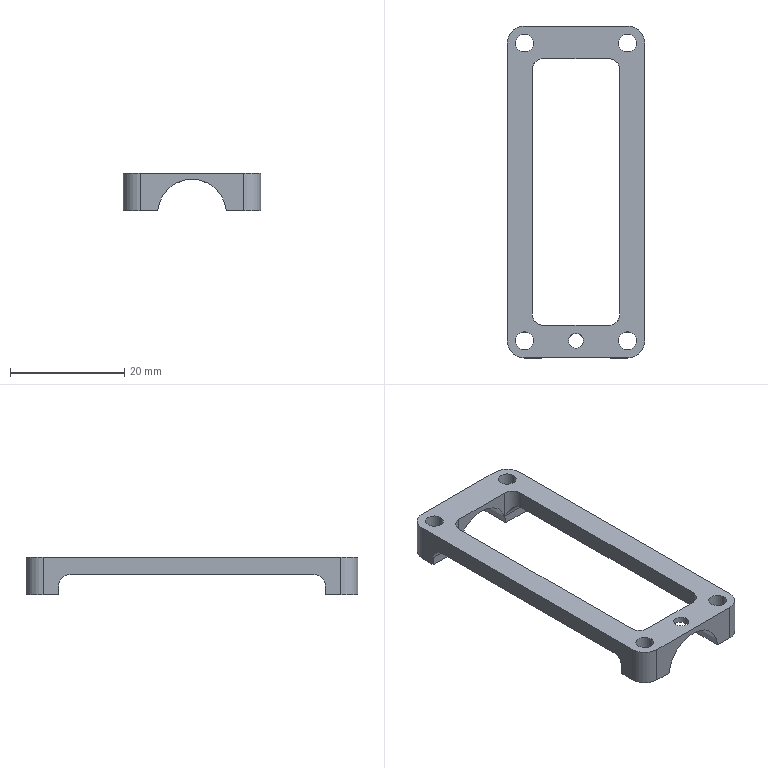Part | SolidWorks | features ICE 2, Extrusion 1, Fillet 1 | 1 solid | 39 faces | box 24 x 58 x 6.5 mm | volume 2190 mm3 | cylinder 24 | plane 15 | commonest cylinder face diameters 3.1 x8 4 x8 6 x4 2.6 x2 12 x2
STEP:
#1=CARTESIAN_POINT('',(1.3,-18.,5.857));
#2=VERTEX_POINT('',#1);
#3=CARTESIAN_POINT('',(-1.3,-18.,5.857));
#4=VERTEX_POINT('',#3);
#5=CARTESIAN_POINT('',(1.3,-18.,5.857));
#6=CARTESIAN_POINT('',(1.3,-18.172,5.857));
#7=CARTESIAN_POINT('',(1.266,-18.341,5.865));
#8=CARTESIAN_POINT('',(1.135,-18.656,5.892));
#9=CARTESIAN_POINT('',(1.039,-18.8,5.911));
#10=CARTESIAN_POINT('',(0.7995,-19.039,5.948));
#11=CARTESIAN_POINT('',(0.6548,-19.136,5.966));
#12=CARTESIAN_POINT('',(0.3421,-19.266,5.992));
#13=CARTESIAN_POINT('',(0.1707,-19.3,6.));
#14=CARTESIAN_POINT('',(-0.08456,-19.3,6.));
#15=CARTESIAN_POINT('',(-0.171,-19.292,5.998));
#16=CARTESIAN_POINT('',(-0.3379,-19.258,5.991));
#17=CARTESIAN_POINT('',(-0.4191,-19.234,5.986));
#18=CARTESIAN_POINT('',(-0.6557,-19.135,5.966));
#19=CARTESIAN_POINT('',(-0.7987,-19.04,5.948));
#20=CARTESIAN_POINT('',(-0.9797,-18.859,5.92));
#21=CARTESIAN_POINT('',(-1.033,-18.793,5.911));
#22=CARTESIAN_POINT('',(-1.127,-18.653,5.893));
#23=CARTESIAN_POINT('',(-1.168,-18.577,5.885));
#24=CARTESIAN_POINT('',(-1.233,-18.42,5.872));
#25=CARTESIAN_POINT('',(-1.258,-18.338,5.867));
#26=CARTESIAN_POINT('',(-1.291,-18.171,5.859));
#27=CARTESIAN_POINT('',(-1.3,-18.085,5.857));
#28=CARTESIAN_POINT('',(-1.3,-18.,5.857));
#29=B_SPLINE_CURVE_WITH_KNOTS('',3,(#5,#6,#7,#8,#9,#10,#11,#12,#13,#14,#15,#16,#17,#18,#19,#20,#21,#22,#23,#24,#25,#26,#27,#28),.UNSPECIFIED.,.F.,.F.,(4,2,2,2,2,2,2,2,2,2,2,4),(0.,0.0005096,0.001019,0.001529,0.002038,0.002293,0.002548,0.003057,0.003312,0.003567,0.003822,0.004076),.UNSPECIFIED.);
#30=EDGE_CURVE('',#2,#4,#29,.T.);
#31=ORIENTED_EDGE('',*,*,#30,.T.);
#32=CARTESIAN_POINT('',(-1.3,-18.,7.));
#33=VERTEX_POINT('',#32);
#34=CARTESIAN_POINT('',(-1.3,-18.,-7.));
#35=DIRECTION('',(0.,0.,1.));
#36=VECTOR('',#35,1000.);
#37=LINE('',#34,#36);
#38=EDGE_CURVE('',#4,#33,#37,.T.);
#39=ORIENTED_EDGE('',*,*,#38,.T.);
#40=CARTESIAN_POINT('',(1.3,-18.,7.));
#41=VERTEX_POINT('',#40);
#42=CARTESIAN_POINT('',(0.,-18.,7.));
#43=DIRECTION('',(0.,0.,1.));
#44=DIRECTION('',(1.,0.,0.));
#45=AXIS2_PLACEMENT_3D('',#42,#43,#44);
#46=CIRCLE('',#45,1.3);
#47=EDGE_CURVE('',#33,#41,#46,.T.);
#48=ORIENTED_EDGE('',*,*,#47,.T.);
#49=CARTESIAN_POINT('',(1.3,-18.,-7.));
#50=DIRECTION('',(0.,0.,1.));
#51=VECTOR('',#50,1000.);
#52=LINE('',#49,#51);
#53=EDGE_CURVE('',#2,#41,#52,.T.);
#54=ORIENTED_EDGE('',*,*,#53,.F.);
#55=EDGE_LOOP('',(#31,#39,#48,#54));
#56=FACE_OUTER_BOUND('',#55,.T.);
#57=CARTESIAN_POINT('',(0.,-18.,-7.));
#58=DIRECTION('',(0.,0.,1.));
#59=DIRECTION('',(1.,0.,0.));
#60=AXIS2_PLACEMENT_3D('',#57,#58,#59);
#61=CYLINDRICAL_SURFACE('',#60,1.3);
#62=ADVANCED_FACE('',(#56),#61,.F.);
#63=CARTESIAN_POINT('',(-10.55,34.,0.5));
#64=VERTEX_POINT('',#63);
#65=CARTESIAN_POINT('',(-7.45,34.,0.5));
#66=VERTEX_POINT('',#65);
#67=CARTESIAN_POINT('',(-9.,34.,0.5));
#68=DIRECTION('',(0.,0.,1.));
#69=DIRECTION('',(-1.,0.,0.));
#70=AXIS2_PLACEMENT_3D('',#67,#68,#69);
#71=CIRCLE('',#70,1.55);
#72=EDGE_CURVE('',#64,#66,#71,.T.);
#73=ORIENTED_EDGE('',*,*,#72,.F.);
#74=CARTESIAN_POINT('',(-10.55,34.,7.));
#75=VERTEX_POINT('',#74);
#76=CARTESIAN_POINT('',(-10.55,34.,-7.));
#77=DIRECTION('',(0.,0.,1.));
#78=VECTOR('',#77,1000.);
#79=LINE('',#76,#78);
#80=EDGE_CURVE('',#64,#75,#79,.T.);
#81=ORIENTED_EDGE('',*,*,#80,.T.);
#82=CARTESIAN_POINT('',(-7.45,34.,7.));
#83=VERTEX_POINT('',#82);
#84=CARTESIAN_POINT('',(-9.,34.,7.));
#85=DIRECTION('',(0.,0.,1.));
#86=DIRECTION('',(1.,0.,0.));
#87=AXIS2_PLACEMENT_3D('',#84,#85,#86);
#88=CIRCLE('',#87,1.55);
#89=EDGE_CURVE('',#75,#83,#88,.T.);
#90=ORIENTED_EDGE('',*,*,#89,.T.);
#91=CARTESIAN_POINT('',(-7.45,34.,-7.));
#92=DIRECTION('',(0.,0.,1.));
#93=VECTOR('',#92,1000.);
#94=LINE('',#91,#93);
#95=EDGE_CURVE('',#66,#83,#94,.T.);
#96=ORIENTED_EDGE('',*,*,#95,.F.);
#97=EDGE_LOOP('',(#73,#81,#90,#96));
#98=FACE_OUTER_BOUND('',#97,.T.);
#99=CARTESIAN_POINT('',(-9.,34.,-7.));
#100=DIRECTION('',(0.,0.,1.));
#101=DIRECTION('',(1.,0.,0.));
#102=AXIS2_PLACEMENT_3D('',#99,#100,#101);
#103=CYLINDRICAL_SURFACE('',#102,1.55);
#104=ADVANCED_FACE('',(#98),#103,.F.);
#105=CARTESIAN_POINT('',(7.45,-18.,0.5));
#106=VERTEX_POINT('',#105);
#107=CARTESIAN_POINT('',(10.55,-18.,0.5));
#108=VERTEX_POINT('',#107);
#109=CARTESIAN_POINT('',(9.,-18.,0.5));
#110=DIRECTION('',(0.,0.,1.));
#111=DIRECTION('',(-1.,0.,0.));
#112=AXIS2_PLACEMENT_3D('',#109,#110,#111);
#113=CIRCLE('',#112,1.55);
#114=EDGE_CURVE('',#106,#108,#113,.T.);
#115=ORIENTED_EDGE('',*,*,#114,.F.);
#116=CARTESIAN_POINT('',(7.45,-18.,7.));
#117=VERTEX_POINT('',#116);
#118=CARTESIAN_POINT('',(7.45,-18.,-7.));
#119=DIRECTION('',(0.,0.,1.));
#120=VECTOR('',#119,1000.);
#121=LINE('',#118,#120);
#122=EDGE_CURVE('',#106,#117,#121,.T.);
#123=ORIENTED_EDGE('',*,*,#122,.T.);
#124=CARTESIAN_POINT('',(10.55,-18.,7.));
#125=VERTEX_POINT('',#124);
#126=CARTESIAN_POINT('',(9.,-18.,7.));
#127=DIRECTION('',(0.,0.,1.));
#128=DIRECTION('',(1.,0.,0.));
#129=AXIS2_PLACEMENT_3D('',#126,#127,#128);
#130=CIRCLE('',#129,1.55);
#131=EDGE_CURVE('',#117,#125,#130,.T.);
#132=ORIENTED_EDGE('',*,*,#131,.T.);
#133=CARTESIAN_POINT('',(10.55,-18.,-7.));
#134=DIRECTION('',(0.,0.,1.));
#135=VECTOR('',#134,1000.);
#136=LINE('',#133,#135);
#137=EDGE_CURVE('',#108,#125,#136,.T.);
#138=ORIENTED_EDGE('',*,*,#137,.F.);
#139=EDGE_LOOP('',(#115,#123,#132,#138));
#140=FACE_OUTER_BOUND('',#139,.T.);
#141=CARTESIAN_POINT('',(9.,-18.,-7.));
#142=DIRECTION('',(0.,0.,1.));
#143=DIRECTION('',(1.,0.,0.));
#144=AXIS2_PLACEMENT_3D('',#141,#142,#143);
#145=CYLINDRICAL_SURFACE('',#144,1.55);
#146=ADVANCED_FACE('',(#140),#145,.F.);
#147=CARTESIAN_POINT('',(7.45,34.,0.5));
#148=VERTEX_POINT('',#147);
#149=CARTESIAN_POINT('',(10.55,34.,0.5));
#150=VERTEX_POINT('',#149);
#151=CARTESIAN_POINT('',(9.,34.,0.5));
#152=DIRECTION('',(0.,0.,1.));
#153=DIRECTION('',(-1.,0.,0.));
#154=AXIS2_PLACEMENT_3D('',#151,#152,#153);
#155=CIRCLE('',#154,1.55);
#156=EDGE_CURVE('',#148,#150,#155,.T.);
#157=ORIENTED_EDGE('',*,*,#156,.F.);
#158=CARTESIAN_POINT('',(7.45,34.,7.));
#159=VERTEX_POINT('',#158);
#160=CARTESIAN_POINT('',(7.45,34.,-7.));
#161=DIRECTION('',(0.,0.,1.));
#162=VECTOR('',#161,1000.);
#163=LINE('',#160,#162);
#164=EDGE_CURVE('',#148,#159,#163,.T.);
#165=ORIENTED_EDGE('',*,*,#164,.T.);
#166=CARTESIAN_POINT('',(10.55,34.,7.));
#167=VERTEX_POINT('',#166);
#168=CARTESIAN_POINT('',(9.,34.,7.));
#169=DIRECTION('',(0.,0.,1.));
#170=DIRECTION('',(1.,0.,0.));
#171=AXIS2_PLACEMENT_3D('',#168,#169,#170);
#172=CIRCLE('',#171,1.55);
#173=EDGE_CURVE('',#159,#167,#172,.T.);
#174=ORIENTED_EDGE('',*,*,#173,.T.);
#175=CARTESIAN_POINT('',(10.55,34.,-7.));
#176=DIRECTION('',(0.,0.,1.));
#177=VECTOR('',#176,1000.);
#178=LINE('',#175,#177);
#179=EDGE_CURVE('',#150,#167,#178,.T.);
#180=ORIENTED_EDGE('',*,*,#179,.F.);
#181=EDGE_LOOP('',(#157,#165,#174,#180));
#182=FACE_OUTER_BOUND('',#181,.T.);
#183=CARTESIAN_POINT('',(9.,34.,-7.));
#184=DIRECTION('',(0.,0.,1.));
#185=DIRECTION('',(1.,0.,0.));
#186=AXIS2_PLACEMENT_3D('',#183,#184,#185);
#187=CYLINDRICAL_SURFACE('',#186,1.55);
#188=ADVANCED_FACE('',(#182),#187,.F.);
#189=CARTESIAN_POINT('',(-10.55,-18.,0.5));
#190=VERTEX_POINT('',#189);
#191=CARTESIAN_POINT('',(-7.45,-18.,0.5));
#192=VERTEX_POINT('',#191);
#193=CARTESIAN_POINT('',(-9.,-18.,0.5));
#194=DIRECTION('',(0.,0.,1.));
#195=DIRECTION('',(-1.,0.,0.));
#196=AXIS2_PLACEMENT_3D('',#193,#194,#195);
#197=CIRCLE('',#196,1.55);
#198=EDGE_CURVE('',#190,#192,#197,.T.);
#199=ORIENTED_EDGE('',*,*,#198,.F.);
#200=CARTESIAN_POINT('',(-10.55,-18.,7.));
#201=VERTEX_POINT('',#200);
#202=CARTESIAN_POINT('',(-10.55,-18.,-7.));
#203=DIRECTION('',(0.,0.,1.));
#204=VECTOR('',#203,1000.);
#205=LINE('',#202,#204);
#206=EDGE_CURVE('',#190,#201,#205,.T.);
#207=ORIENTED_EDGE('',*,*,#206,.T.);
#208=CARTESIAN_POINT('',(-7.45,-18.,7.));
#209=VERTEX_POINT('',#208);
#210=CARTESIAN_POINT('',(-9.,-18.,7.));
#211=DIRECTION('',(0.,0.,1.));
#212=DIRECTION('',(1.,0.,0.));
#213=AXIS2_PLACEMENT_3D('',#210,#211,#212);
#214=CIRCLE('',#213,1.55);
#215=EDGE_CURVE('',#201,#209,#214,.T.);
#216=ORIENTED_EDGE('',*,*,#215,.T.);
#217=CARTESIAN_POINT('',(-7.45,-18.,-7.));
#218=DIRECTION('',(0.,0.,1.));
#219=VECTOR('',#218,1000.);
#220=LINE('',#217,#219);
#221=EDGE_CURVE('',#192,#209,#220,.T.);
#222=ORIENTED_EDGE('',*,*,#221,.F.);
#223=EDGE_LOOP('',(#199,#207,#216,#222));
#224=FACE_OUTER_BOUND('',#223,.T.);
#225=CARTESIAN_POINT('',(-9.,-18.,-7.));
#226=DIRECTION('',(0.,0.,1.));
#227=DIRECTION('',(1.,0.,0.));
#228=AXIS2_PLACEMENT_3D('',#225,#226,#227);
#229=CYLINDRICAL_SURFACE('',#228,1.55);
#230=ADVANCED_FACE('',(#224),#229,.F.);
#231=CARTESIAN_POINT('',(12.,-15.317,2.));
#232=VERTEX_POINT('',#231);
#233=CARTESIAN_POINT('',(12.,-15.317,0.5));
#234=VERTEX_POINT('',#233);
#235=CARTESIAN_POINT('',(12.,-15.317,0.));
#236=DIRECTION('',(0.,0.,-1.));
#237=VECTOR('',#236,1000.);
#238=LINE('',#235,#237);
#239=EDGE_CURVE('',#232,#234,#238,.T.);
#240=ORIENTED_EDGE('',*,*,#239,.F.);
#241=CARTESIAN_POINT('',(12.,-13.317,4.));
#242=VERTEX_POINT('',#241);
#243=CARTESIAN_POINT('',(12.,-13.317,2.));
#244=DIRECTION('',(-1.,0.,0.));
#245=DIRECTION('',(0.,-1.,0.));
#246=AXIS2_PLACEMENT_3D('',#243,#244,#245);
#247=CIRCLE('',#246,2.);
#248=EDGE_CURVE('',#232,#242,#247,.T.);
#249=ORIENTED_EDGE('',*,*,#248,.T.);
#250=CARTESIAN_POINT('',(12.,29.317,4.));
#251=VERTEX_POINT('',#250);
#252=CARTESIAN_POINT('',(12.,0.,4.));
#253=DIRECTION('',(0.,-1.,0.));
#254=VECTOR('',#253,1000.);
#255=LINE('',#252,#254);
#256=EDGE_CURVE('',#251,#242,#255,.T.);
#257=ORIENTED_EDGE('',*,*,#256,.F.);
#258=CARTESIAN_POINT('',(12.,31.317,2.));
#259=VERTEX_POINT('',#258);
#260=CARTESIAN_POINT('',(12.,29.317,2.));
#261=DIRECTION('',(-1.,0.,0.));
#262=DIRECTION('',(0.,-1.,0.));
#263=AXIS2_PLACEMENT_3D('',#260,#261,#262);
#264=CIRCLE('',#263,2.);
#265=EDGE_CURVE('',#251,#259,#264,.T.);
#266=ORIENTED_EDGE('',*,*,#265,.T.);
#267=CARTESIAN_POINT('',(12.,31.317,0.5));
#268=VERTEX_POINT('',#267);
#269=CARTESIAN_POINT('',(12.,31.317,0.));
#270=DIRECTION('',(0.,0.,-1.));
#271=VECTOR('',#270,1000.);
#272=LINE('',#269,#271);
#273=EDGE_CURVE('',#259,#268,#272,.T.);
#274=ORIENTED_EDGE('',*,*,#273,.T.);
#275=CARTESIAN_POINT('',(12.,34.,0.5));
#276=VERTEX_POINT('',#275);
#277=CARTESIAN_POINT('',(12.,37.,0.5));
#278=DIRECTION('',(0.,-1.,0.));
#279=VECTOR('',#278,1000.);
#280=LINE('',#277,#279);
#281=EDGE_CURVE('',#276,#268,#280,.T.);
#282=ORIENTED_EDGE('',*,*,#281,.F.);
#283=CARTESIAN_POINT('',(12.,34.,7.));
#284=VERTEX_POINT('',#283);
#285=CARTESIAN_POINT('',(12.,34.,-7.));
#286=DIRECTION('',(0.,0.,1.));
#287=VECTOR('',#286,1000.);
#288=LINE('',#285,#287);
#289=EDGE_CURVE('',#276,#284,#288,.T.);
#290=ORIENTED_EDGE('',*,*,#289,.T.);
#291=CARTESIAN_POINT('',(12.,-18.,7.));
#292=VERTEX_POINT('',#291);
#293=CARTESIAN_POINT('',(12.,0.,7.));
#294=DIRECTION('',(0.,-1.,0.));
#295=VECTOR('',#294,1000.);
#296=LINE('',#293,#295);
#297=EDGE_CURVE('',#284,#292,#296,.T.);
#298=ORIENTED_EDGE('',*,*,#297,.T.);
#299=CARTESIAN_POINT('',(12.,-18.,0.5));
#300=VERTEX_POINT('',#299);
#301=CARTESIAN_POINT('',(12.,-18.,-7.));
#302=DIRECTION('',(0.,0.,1.));
#303=VECTOR('',#302,1000.);
#304=LINE('',#301,#303);
#305=EDGE_CURVE('',#300,#292,#304,.T.);
#306=ORIENTED_EDGE('',*,*,#305,.F.);
#307=CARTESIAN_POINT('',(12.,37.,0.5));
#308=DIRECTION('',(0.,-1.,0.));
#309=VECTOR('',#308,1000.);
#310=LINE('',#307,#309);
#311=EDGE_CURVE('',#234,#300,#310,.T.);
#312=ORIENTED_EDGE('',*,*,#311,.F.);
#313=EDGE_LOOP('',(#240,#249,#257,#266,#274,#282,#290,#298,#306,#312));
#314=FACE_OUTER_BOUND('',#313,.T.);
#315=CARTESIAN_POINT('',(12.,0.,-7.));
#316=DIRECTION('',(-1.,0.,0.));
#317=DIRECTION('',(0.,-1.,0.));
#318=AXIS2_PLACEMENT_3D('',#315,#316,#317);
#319=PLANE('',#318);
#320=ADVANCED_FACE('',(#314),#319,.F.);
#321=CARTESIAN_POINT('',(-12.,29.317,4.));
#322=VERTEX_POINT('',#321);
#323=CARTESIAN_POINT('',(-12.,-13.317,4.));
#324=VERTEX_POINT('',#323);
#325=CARTESIAN_POINT('',(-12.,0.,4.));
#326=DIRECTION('',(0.,-1.,0.));
#327=VECTOR('',#326,1000.);
#328=LINE('',#325,#327);
#329=EDGE_CURVE('',#322,#324,#328,.T.);
#330=ORIENTED_EDGE('',*,*,#329,.T.);
#331=CARTESIAN_POINT('',(-12.,-15.317,2.));
#332=VERTEX_POINT('',#331);
#333=CARTESIAN_POINT('',(-12.,-13.317,2.));
#334=DIRECTION('',(1.,0.,0.));
#335=DIRECTION('',(0.,1.,0.));
#336=AXIS2_PLACEMENT_3D('',#333,#334,#335);
#337=CIRCLE('',#336,2.);
#338=EDGE_CURVE('',#324,#332,#337,.T.);
#339=ORIENTED_EDGE('',*,*,#338,.T.);
#340=CARTESIAN_POINT('',(-12.,-15.317,0.5));
#341=VERTEX_POINT('',#340);
#342=CARTESIAN_POINT('',(-12.,-15.317,0.));
#343=DIRECTION('',(0.,0.,-1.));
#344=VECTOR('',#343,1000.);
#345=LINE('',#342,#344);
#346=EDGE_CURVE('',#332,#341,#345,.T.);
#347=ORIENTED_EDGE('',*,*,#346,.T.);
#348=CARTESIAN_POINT('',(-12.,-18.,0.5));
#349=VERTEX_POINT('',#348);
#350=CARTESIAN_POINT('',(-12.,37.,0.5));
#351=DIRECTION('',(0.,-1.,0.));
#352=VECTOR('',#351,1000.);
#353=LINE('',#350,#352);
#354=EDGE_CURVE('',#341,#349,#353,.T.);
#355=ORIENTED_EDGE('',*,*,#354,.T.);
#356=CARTESIAN_POINT('',(-12.,-18.,7.));
#357=VERTEX_POINT('',#356);
#358=CARTESIAN_POINT('',(-12.,-18.,-7.));
#359=DIRECTION('',(0.,0.,1.));
#360=VECTOR('',#359,1000.);
#361=LINE('',#358,#360);
#362=EDGE_CURVE('',#349,#357,#361,.T.);
#363=ORIENTED_EDGE('',*,*,#362,.T.);
#364=CARTESIAN_POINT('',(-12.,34.,7.));
#365=VERTEX_POINT('',#364);
#366=CARTESIAN_POINT('',(-12.,0.,7.));
#367=DIRECTION('',(0.,1.,0.));
#368=VECTOR('',#367,1000.);
#369=LINE('',#366,#368);
#370=EDGE_CURVE('',#357,#365,#369,.T.);
#371=ORIENTED_EDGE('',*,*,#370,.T.);
#372=CARTESIAN_POINT('',(-12.,34.,0.5));
#373=VERTEX_POINT('',#372);
#374=CARTESIAN_POINT('',(-12.,34.,-7.));
#375=DIRECTION('',(0.,0.,1.));
#376=VECTOR('',#375,1000.);
#377=LINE('',#374,#376);
#378=EDGE_CURVE('',#373,#365,#377,.T.);
#379=ORIENTED_EDGE('',*,*,#378,.F.);
#380=CARTESIAN_POINT('',(-12.,31.317,0.5));
#381=VERTEX_POINT('',#380);
#382=CARTESIAN_POINT('',(-12.,37.,0.5));
#383=DIRECTION('',(0.,-1.,0.));
#384=VECTOR('',#383,1000.);
#385=LINE('',#382,#384);
#386=EDGE_CURVE('',#373,#381,#385,.T.);
#387=ORIENTED_EDGE('',*,*,#386,.T.);
#388=CARTESIAN_POINT('',(-12.,31.317,2.));
#389=VERTEX_POINT('',#388);
#390=CARTESIAN_POINT('',(-12.,31.317,0.));
#391=DIRECTION('',(0.,0.,-1.));
#392=VECTOR('',#391,1000.);
#393=LINE('',#390,#392);
#394=EDGE_CURVE('',#389,#381,#393,.T.);
#395=ORIENTED_EDGE('',*,*,#394,.F.);
#396=CARTESIAN_POINT('',(-12.,29.317,2.));
#397=DIRECTION('',(1.,0.,0.));
#398=DIRECTION('',(0.,1.,0.));
#399=AXIS2_PLACEMENT_3D('',#396,#397,#398);
#400=CIRCLE('',#399,2.);
#401=EDGE_CURVE('',#389,#322,#400,.T.);
#402=ORIENTED_EDGE('',*,*,#401,.T.);
#403=EDGE_LOOP('',(#330,#339,#347,#355,#363,#371,#379,#387,#395,#402));
#404=FACE_OUTER_BOUND('',#403,.T.);
#405=CARTESIAN_POINT('',(-12.,0.,-7.));
#406=DIRECTION('',(1.,0.,0.));
#407=DIRECTION('',(0.,1.,0.));
#408=AXIS2_PLACEMENT_3D('',#405,#406,#407);
#409=PLANE('',#408);
#410=ADVANCED_FACE('',(#404),#409,.F.);
#411=CARTESIAN_POINT('',(-7.658,29.317,4.));
#412=VERTEX_POINT('',#411);
#413=CARTESIAN_POINT('',(-7.658,-13.317,4.));
#414=VERTEX_POINT('',#413);
#415=CARTESIAN_POINT('',(-7.658,0.,4.));
#416=DIRECTION('',(0.,-1.,0.));
#417=VECTOR('',#416,1000.);
#418=LINE('',#415,#417);
#419=EDGE_CURVE('',#412,#414,#418,.T.);
#420=ORIENTED_EDGE('',*,*,#419,.F.);
#421=CARTESIAN_POINT('',(-7.658,29.317,7.));
#422=VERTEX_POINT('',#421);
#423=CARTESIAN_POINT('',(-7.658,29.317,-7.));
#424=DIRECTION('',(0.,0.,1.));
#425=VECTOR('',#424,1000.);
#426=LINE('',#423,#425);
#427=EDGE_CURVE('',#412,#422,#426,.T.);
#428=ORIENTED_EDGE('',*,*,#427,.T.);
#429=CARTESIAN_POINT('',(-7.658,-13.317,7.));
#430=VERTEX_POINT('',#429);
#431=CARTESIAN_POINT('',(-7.658,0.,7.));
#432=DIRECTION('',(0.,-1.,0.));
#433=VECTOR('',#432,1000.);
#434=LINE('',#431,#433);
#435=EDGE_CURVE('',#422,#430,#434,.T.);
#436=ORIENTED_EDGE('',*,*,#435,.T.);
#437=CARTESIAN_POINT('',(-7.658,-13.317,4.));
#438=DIRECTION('',(0.,0.,-1.));
#439=VECTOR('',#438,1000.);
#440=LINE('',#437,#439);
#441=EDGE_CURVE('',#430,#414,#440,.T.);
#442=ORIENTED_EDGE('',*,*,#441,.T.);
#443=EDGE_LOOP('',(#420,#428,#436,#442));
#444=FACE_OUTER_BOUND('',#443,.T.);
#445=CARTESIAN_POINT('',(-7.658,0.,-7.));
#446=DIRECTION('',(-1.,0.,0.));
#447=DIRECTION('',(0.,-1.,0.));
#448=AXIS2_PLACEMENT_3D('',#445,#446,#447);
#449=PLANE('',#448);
#450=ADVANCED_FACE('',(#444),#449,.F.);
#451=CARTESIAN_POINT('',(7.658,29.317,7.));
#452=VERTEX_POINT('',#451);
#453=CARTESIAN_POINT('',(7.658,-13.317,7.));
#454=VERTEX_POINT('',#453);
#455=CARTESIAN_POINT('',(7.658,0.,7.));
#456=DIRECTION('',(0.,-1.,0.));
#457=VECTOR('',#456,1000.);
#458=LINE('',#455,#457);
#459=EDGE_CURVE('',#452,#454,#458,.T.);
#460=ORIENTED_EDGE('',*,*,#459,.F.);
#461=CARTESIAN_POINT('',(7.658,29.317,4.));
#462=VERTEX_POINT('',#461);
#463=CARTESIAN_POINT('',(7.658,29.317,4.));
#464=DIRECTION('',(0.,0.,-1.));
#465=VECTOR('',#464,1000.);
#466=LINE('',#463,#465);
#467=EDGE_CURVE('',#452,#462,#466,.T.);
#468=ORIENTED_EDGE('',*,*,#467,.T.);
#469=CARTESIAN_POINT('',(7.658,-13.317,4.));
#470=VERTEX_POINT('',#469);
#471=CARTESIAN_POINT('',(7.658,0.,4.));
#472=DIRECTION('',(0.,-1.,0.));
#473=VECTOR('',#472,1000.);
#474=LINE('',#471,#473);
#475=EDGE_CURVE('',#462,#470,#474,.T.);
#476=ORIENTED_EDGE('',*,*,#475,.T.);
#477=CARTESIAN_POINT('',(7.658,-13.317,-7.));
#478=DIRECTION('',(0.,0.,1.));
#479=VECTOR('',#478,1000.);
#480=LINE('',#477,#479);
#481=EDGE_CURVE('',#470,#454,#480,.T.);
#482=ORIENTED_EDGE('',*,*,#481,.T.);
#483=EDGE_LOOP('',(#460,#468,#476,#482));
#484=FACE_OUTER_BOUND('',#483,.T.);
#485=CARTESIAN_POINT('',(7.658,0.,-7.));
#486=DIRECTION('',(-1.,0.,0.));
#487=DIRECTION('',(0.,-1.,0.));
#488=AXIS2_PLACEMENT_3D('',#485,#486,#487);
#489=PLANE('',#488);
#490=ADVANCED_FACE('',(#484),#489,.T.);
#491=CARTESIAN_POINT('',(9.,-18.,0.5));
#492=DIRECTION('',(0.,0.,1.));
#493=DIRECTION('',(-1.,0.,0.));
#494=AXIS2_PLACEMENT_3D('',#491,#492,#493);
#495=CIRCLE('',#494,1.55);
#496=EDGE_CURVE('',#108,#106,#495,.T.);
#497=ORIENTED_EDGE('',*,*,#496,.T.);
#498=ORIENTED_EDGE('',*,*,#114,.T.);
#499=EDGE_LOOP('',(#497,#498));
#500=FACE_BOUND('',#499,.T.);
#501=CARTESIAN_POINT('',(5.979,-15.317,0.5));
#502=VERTEX_POINT('',#501);
#503=CARTESIAN_POINT('',(0.,-15.317,0.5));
#504=DIRECTION('',(1.,0.,0.));
#505=VECTOR('',#504,1000.);
#506=LINE('',#503,#505);
#507=EDGE_CURVE('',#502,#234,#506,.T.);
#508=ORIENTED_EDGE('',*,*,#507,.T.);
#509=ORIENTED_EDGE('',*,*,#311,.T.);
#510=CARTESIAN_POINT('',(9.,-21.,0.5));
#511=VERTEX_POINT('',#510);
#512=CARTESIAN_POINT('',(9.,-18.,0.5));
#513=DIRECTION('',(0.,0.,1.));
#514=DIRECTION('',(-1.,0.,0.));
#515=AXIS2_PLACEMENT_3D('',#512,#513,#514);
#516=CIRCLE('',#515,3.);
#517=EDGE_CURVE('',#511,#300,#516,.T.);
#518=ORIENTED_EDGE('',*,*,#517,.F.);
#519=CARTESIAN_POINT('',(5.979,-21.,0.5));
#520=VERTEX_POINT('',#519);
#521=CARTESIAN_POINT('',(0.,-21.,0.5));
#522=DIRECTION('',(1.,0.,0.));
#523=VECTOR('',#522,1000.);
#524=LINE('',#521,#523);
#525=EDGE_CURVE('',#520,#511,#524,.T.);
#526=ORIENTED_EDGE('',*,*,#525,.F.);
#527=CARTESIAN_POINT('',(5.979,37.,0.5));
#528=DIRECTION('',(0.,-1.,0.));
#529=VECTOR('',#528,1000.);
#530=LINE('',#527,#529);
#531=EDGE_CURVE('',#502,#520,#530,.T.);
#532=ORIENTED_EDGE('',*,*,#531,.F.);
#533=EDGE_LOOP('',(#508,#509,#518,#526,#532));
#534=FACE_OUTER_BOUND('',#533,.T.);
#535=CARTESIAN_POINT('',(0.,37.,0.5));
#536=DIRECTION('',(0.,0.,-1.));
#537=DIRECTION('',(-1.,0.,0.));
#538=AXIS2_PLACEMENT_3D('',#535,#536,#537);
#539=PLANE('',#538);
#540=ADVANCED_FACE('',(#500,#534),#539,.T.);
#541=CARTESIAN_POINT('',(-9.,-18.,0.5));
#542=DIRECTION('',(0.,0.,1.));
#543=DIRECTION('',(-1.,0.,0.));
#544=AXIS2_PLACEMENT_3D('',#541,#542,#543);
#545=CIRCLE('',#544,1.55);
#546=EDGE_CURVE('',#192,#190,#545,.T.);
#547=ORIENTED_EDGE('',*,*,#546,.T.);
#548=ORIENTED_EDGE('',*,*,#198,.T.);
#549=EDGE_LOOP('',(#547,#548));
#550=FACE_BOUND('',#549,.T.);
#551=ORIENTED_EDGE('',*,*,#354,.F.);
#552=CARTESIAN_POINT('',(-5.979,-15.317,0.5));
#553=VERTEX_POINT('',#552);
#554=CARTESIAN_POINT('',(0.,-15.317,0.5));
#555=DIRECTION('',(1.,0.,0.));
#556=VECTOR('',#555,1000.);
#557=LINE('',#554,#556);
#558=EDGE_CURVE('',#341,#553,#557,.T.);
#559=ORIENTED_EDGE('',*,*,#558,.T.);
#560=CARTESIAN_POINT('',(-5.979,-21.,0.5));
#561=VERTEX_POINT('',#560);
#562=CARTESIAN_POINT('',(-5.979,37.,0.5));
#563=DIRECTION('',(0.,-1.,0.));
#564=VECTOR('',#563,1000.);
#565=LINE('',#562,#564);
#566=EDGE_CURVE('',#553,#561,#565,.T.);
#567=ORIENTED_EDGE('',*,*,#566,.T.);
#568=CARTESIAN_POINT('',(-9.,-21.,0.5));
#569=VERTEX_POINT('',#568);
#570=CARTESIAN_POINT('',(0.,-21.,0.5));
#571=DIRECTION('',(1.,0.,0.));
#572=VECTOR('',#571,1000.);
#573=LINE('',#570,#572);
#574=EDGE_CURVE('',#569,#561,#573,.T.);
#575=ORIENTED_EDGE('',*,*,#574,.F.);
#576=CARTESIAN_POINT('',(-9.,-18.,0.5));
#577=DIRECTION('',(0.,0.,1.));
#578=DIRECTION('',(-1.,0.,0.));
#579=AXIS2_PLACEMENT_3D('',#576,#577,#578);
#580=CIRCLE('',#579,3.);
#581=EDGE_CURVE('',#349,#569,#580,.T.);
#582=ORIENTED_EDGE('',*,*,#581,.F.);
#583=EDGE_LOOP('',(#551,#559,#567,#575,#582));
#584=FACE_OUTER_BOUND('',#583,.T.);
#585=CARTESIAN_POINT('',(0.,37.,0.5));
#586=DIRECTION('',(0.,0.,-1.));
#587=DIRECTION('',(-1.,0.,0.));
#588=AXIS2_PLACEMENT_3D('',#585,#586,#587);
#589=PLANE('',#588);
#590=ADVANCED_FACE('',(#550,#584),#589,.T.);
#591=CARTESIAN_POINT('',(9.,-21.,7.));
#592=VERTEX_POINT('',#591);
#593=CARTESIAN_POINT('',(9.,-21.,-7.));
#594=DIRECTION('',(0.,0.,1.));
#595=VECTOR('',#594,1000.);
#596=LINE('',#593,#595);
#597=EDGE_CURVE('',#511,#592,#596,.T.);
#598=ORIENTED_EDGE('',*,*,#597,.F.);
#599=ORIENTED_EDGE('',*,*,#517,.T.);
#600=ORIENTED_EDGE('',*,*,#305,.T.);
#601=CARTESIAN_POINT('',(9.,-18.,7.));
#602=DIRECTION('',(0.,0.,1.));
#603=DIRECTION('',(1.,0.,0.));
#604=AXIS2_PLACEMENT_3D('',#601,#602,#603);
#605=CIRCLE('',#604,3.);
#606=EDGE_CURVE('',#592,#292,#605,.T.);
#607=ORIENTED_EDGE('',*,*,#606,.F.);
#608=EDGE_LOOP('',(#598,#599,#600,#607));
#609=FACE_OUTER_BOUND('',#608,.T.);
#610=CARTESIAN_POINT('',(9.,-18.,-7.));
#611=DIRECTION('',(0.,0.,1.));
#612=DIRECTION('',(1.,0.,0.));
#613=AXIS2_PLACEMENT_3D('',#610,#611,#612);
#614=CYLINDRICAL_SURFACE('',#613,3.);
#615=ADVANCED_FACE('',(#609),#614,.T.);
#616=ORIENTED_EDGE('',*,*,#525,.T.);
#617=ORIENTED_EDGE('',*,*,#597,.T.);
#618=CARTESIAN_POINT('',(-9.,-21.,7.));
#619=VERTEX_POINT('',#618);
#620=CARTESIAN_POINT('',(0.,-21.,7.));
#621=DIRECTION('',(-1.,0.,0.));
#622=VECTOR('',#621,1000.);
#623=LINE('',#620,#622);
#624=EDGE_CURVE('',#592,#619,#623,.T.);
#625=ORIENTED_EDGE('',*,*,#624,.T.);
#626=CARTESIAN_POINT('',(-9.,-21.,-7.));
#627=DIRECTION('',(0.,0.,1.));
#628=VECTOR('',#627,1000.);
#629=LINE('',#626,#628);
#630=EDGE_CURVE('',#569,#619,#629,.T.);
#631=ORIENTED_EDGE('',*,*,#630,.F.);
#632=ORIENTED_EDGE('',*,*,#574,.T.);
#633=CARTESIAN_POINT('',(0.,-21.,0.));
#634=DIRECTION('',(0.,-1.,0.));
#635=DIRECTION('',(0.,0.,-1.));
#636=AXIS2_PLACEMENT_3D('',#633,#634,#635);
#637=CIRCLE('',#636,6.);
#638=EDGE_CURVE('',#520,#561,#637,.T.);
#639=ORIENTED_EDGE('',*,*,#638,.F.);
#640=EDGE_LOOP('',(#616,#617,#625,#631,#632,#639));
#641=FACE_OUTER_BOUND('',#640,.T.);
#642=CARTESIAN_POINT('',(0.,-21.,-7.));
#643=DIRECTION('',(0.,1.,0.));
#644=DIRECTION('',(0.,0.,1.));
#645=AXIS2_PLACEMENT_3D('',#642,#643,#644);
#646=PLANE('',#645);
#647=ADVANCED_FACE('',(#641),#646,.F.);
#648=ORIENTED_EDGE('',*,*,#362,.F.);
#649=ORIENTED_EDGE('',*,*,#581,.T.);
#650=ORIENTED_EDGE('',*,*,#630,.T.);
#651=CARTESIAN_POINT('',(-9.,-18.,7.));
#652=DIRECTION('',(0.,0.,1.));
#653=DIRECTION('',(1.,0.,0.));
#654=AXIS2_PLACEMENT_3D('',#651,#652,#653);
#655=CIRCLE('',#654,3.);
#656=EDGE_CURVE('',#357,#619,#655,.T.);
#657=ORIENTED_EDGE('',*,*,#656,.F.);
#658=EDGE_LOOP('',(#648,#649,#650,#657));
#659=FACE_OUTER_BOUND('',#658,.T.);
#660=CARTESIAN_POINT('',(-9.,-18.,-7.));
#661=DIRECTION('',(0.,0.,1.));
#662=DIRECTION('',(1.,0.,0.));
#663=AXIS2_PLACEMENT_3D('',#660,#661,#662);
#664=CYLINDRICAL_SURFACE('',#663,3.);
#665=ADVANCED_FACE('',(#659),#664,.T.);
#666=CARTESIAN_POINT('',(-9.,37.,0.5));
#667=VERTEX_POINT('',#666);
#668=CARTESIAN_POINT('',(-9.,37.,7.));
#669=VERTEX_POINT('',#668);
#670=CARTESIAN_POINT('',(-9.,37.,-7.));
#671=DIRECTION('',(0.,0.,1.));
#672=VECTOR('',#671,1000.);
#673=LINE('',#670,#672);
#674=EDGE_CURVE('',#667,#669,#673,.T.);
#675=ORIENTED_EDGE('',*,*,#674,.F.);
#676=CARTESIAN_POINT('',(-9.,34.,0.5));
#677=DIRECTION('',(0.,0.,1.));
#678=DIRECTION('',(-1.,0.,0.));
#679=AXIS2_PLACEMENT_3D('',#676,#677,#678);
#680=CIRCLE('',#679,3.);
#681=EDGE_CURVE('',#667,#373,#680,.T.);
#682=ORIENTED_EDGE('',*,*,#681,.T.);
#683=ORIENTED_EDGE('',*,*,#378,.T.);
#684=CARTESIAN_POINT('',(-9.,34.,7.));
#685=DIRECTION('',(0.,0.,1.));
#686=DIRECTION('',(1.,0.,0.));
#687=AXIS2_PLACEMENT_3D('',#684,#685,#686);
#688=CIRCLE('',#687,3.);
#689=EDGE_CURVE('',#669,#365,#688,.T.);
#690=ORIENTED_EDGE('',*,*,#689,.F.);
#691=EDGE_LOOP('',(#675,#682,#683,#690));
#692=FACE_OUTER_BOUND('',#691,.T.);
#693=CARTESIAN_POINT('',(-9.,34.,-7.));
#694=DIRECTION('',(0.,0.,1.));
#695=DIRECTION('',(1.,0.,0.));
#696=AXIS2_PLACEMENT_3D('',#693,#694,#695);
#697=CYLINDRICAL_SURFACE('',#696,3.);
#698=ADVANCED_FACE('',(#692),#697,.T.);
#699=CARTESIAN_POINT('',(5.979,37.,0.5));
#700=VERTEX_POINT('',#699);
#701=CARTESIAN_POINT('',(9.,37.,0.5));
#702=VERTEX_POINT('',#701);
#703=CARTESIAN_POINT('',(0.,37.,0.5));
#704=DIRECTION('',(1.,0.,0.));
#705=VECTOR('',#704,1000.);
#706=LINE('',#703,#705);
#707=EDGE_CURVE('',#700,#702,#706,.T.);
#708=ORIENTED_EDGE('',*,*,#707,.F.);
#709=CARTESIAN_POINT('',(-5.979,37.,0.5));
#710=VERTEX_POINT('',#709);
#711=CARTESIAN_POINT('',(0.,37.,0.));
#712=DIRECTION('',(0.,-1.,0.));
#713=DIRECTION('',(0.,0.,-1.));
#714=AXIS2_PLACEMENT_3D('',#711,#712,#713);
#715=CIRCLE('',#714,6.);
#716=EDGE_CURVE('',#700,#710,#715,.T.);
#717=ORIENTED_EDGE('',*,*,#716,.T.);
#718=CARTESIAN_POINT('',(0.,37.,0.5));
#719=DIRECTION('',(1.,0.,0.));
#720=VECTOR('',#719,1000.);
#721=LINE('',#718,#720);
#722=EDGE_CURVE('',#667,#710,#721,.T.);
#723=ORIENTED_EDGE('',*,*,#722,.F.);
#724=ORIENTED_EDGE('',*,*,#674,.T.);
#725=CARTESIAN_POINT('',(9.,37.,7.));
#726=VERTEX_POINT('',#725);
#727=CARTESIAN_POINT('',(0.,37.,7.));
#728=DIRECTION('',(1.,0.,0.));
#729=VECTOR('',#728,1000.);
#730=LINE('',#727,#729);
#731=EDGE_CURVE('',#669,#726,#730,.T.);
#732=ORIENTED_EDGE('',*,*,#731,.T.);
#733=CARTESIAN_POINT('',(9.,37.,-7.));
#734=DIRECTION('',(0.,0.,1.));
#735=VECTOR('',#734,1000.);
#736=LINE('',#733,#735);
#737=EDGE_CURVE('',#702,#726,#736,.T.);
#738=ORIENTED_EDGE('',*,*,#737,.F.);
#739=EDGE_LOOP('',(#708,#717,#723,#724,#732,#738));
#740=FACE_OUTER_BOUND('',#739,.T.);
#741=CARTESIAN_POINT('',(0.,37.,-7.));
#742=DIRECTION('',(0.,-1.,0.));
#743=DIRECTION('',(0.,0.,-1.));
#744=AXIS2_PLACEMENT_3D('',#741,#742,#743);
#745=PLANE('',#744);
#746=ADVANCED_FACE('',(#740),#745,.F.);
#747=CARTESIAN_POINT('',(5.658,-15.317,7.));
#748=VERTEX_POINT('',#747);
#749=CARTESIAN_POINT('',(5.658,-15.317,2.));
#750=VERTEX_POINT('',#749);
#751=CARTESIAN_POINT('',(5.658,-15.317,-7.));
#752=DIRECTION('',(0.,0.,-1.));
#753=VECTOR('',#752,1000.);
#754=LINE('',#751,#753);
#755=EDGE_CURVE('',#748,#750,#754,.T.);
#756=ORIENTED_EDGE('',*,*,#755,.T.);
#757=CARTESIAN_POINT('',(0.,-15.317,2.));
#758=DIRECTION('',(1.,0.,0.));
#759=VECTOR('',#758,1000.);
#760=LINE('',#757,#759);
#761=EDGE_CURVE('',#750,#232,#760,.T.);
#762=ORIENTED_EDGE('',*,*,#761,.T.);
#763=ORIENTED_EDGE('',*,*,#239,.T.);
#764=ORIENTED_EDGE('',*,*,#507,.F.);
#765=CARTESIAN_POINT('',(0.,-15.317,0.));
#766=DIRECTION('',(0.,-1.,0.));
#767=DIRECTION('',(1.,0.,0.));
#768=AXIS2_PLACEMENT_3D('',#765,#766,#767);
#769=CIRCLE('',#768,6.);
#770=EDGE_CURVE('',#502,#553,#769,.T.);
#771=ORIENTED_EDGE('',*,*,#770,.T.);
#772=ORIENTED_EDGE('',*,*,#558,.F.);
#773=ORIENTED_EDGE('',*,*,#346,.F.);
#774=CARTESIAN_POINT('',(-5.658,-15.317,2.));
#775=VERTEX_POINT('',#774);
#776=CARTESIAN_POINT('',(0.,-15.317,2.));
#777=DIRECTION('',(1.,0.,0.));
#778=VECTOR('',#777,1000.);
#779=LINE('',#776,#778);
#780=EDGE_CURVE('',#332,#775,#779,.T.);
#781=ORIENTED_EDGE('',*,*,#780,.T.);
#782=CARTESIAN_POINT('',(-5.658,-15.317,7.));
#783=VERTEX_POINT('',#782);
#784=CARTESIAN_POINT('',(-5.658,-15.317,7.));
#785=DIRECTION('',(0.,0.,1.));
#786=VECTOR('',#785,1000.);
#787=LINE('',#784,#786);
#788=EDGE_CURVE('',#775,#783,#787,.T.);
#789=ORIENTED_EDGE('',*,*,#788,.T.);
#790=CARTESIAN_POINT('',(0.,-15.317,7.));
#791=DIRECTION('',(1.,0.,0.));
#792=VECTOR('',#791,1000.);
#793=LINE('',#790,#792);
#794=EDGE_CURVE('',#783,#748,#793,.T.);
#795=ORIENTED_EDGE('',*,*,#794,.T.);
#796=EDGE_LOOP('',(#756,#762,#763,#764,#771,#772,#773,#781,#789,#795));
#797=FACE_OUTER_BOUND('',#796,.T.);
#798=CARTESIAN_POINT('',(0.,-15.317,-7.));
#799=DIRECTION('',(0.,-1.,0.));
#800=DIRECTION('',(1.,0.,0.));
#801=AXIS2_PLACEMENT_3D('',#798,#799,#800);
#802=PLANE('',#801);
#803=ADVANCED_FACE('',(#797),#802,.F.);
#804=ORIENTED_EDGE('',*,*,#206,.F.);
#805=ORIENTED_EDGE('',*,*,#546,.F.);
#806=ORIENTED_EDGE('',*,*,#221,.T.);
#807=CARTESIAN_POINT('',(-9.,-18.,7.));
#808=DIRECTION('',(0.,0.,1.));
#809=DIRECTION('',(1.,0.,0.));
#810=AXIS2_PLACEMENT_3D('',#807,#808,#809);
#811=CIRCLE('',#810,1.55);
#812=EDGE_CURVE('',#209,#201,#811,.T.);
#813=ORIENTED_EDGE('',*,*,#812,.T.);
#814=EDGE_LOOP('',(#804,#805,#806,#813));
#815=FACE_OUTER_BOUND('',#814,.T.);
#816=CARTESIAN_POINT('',(-9.,-18.,-7.));
#817=DIRECTION('',(0.,0.,1.));
#818=DIRECTION('',(1.,0.,0.));
#819=AXIS2_PLACEMENT_3D('',#816,#817,#818);
#820=CYLINDRICAL_SURFACE('',#819,1.55);
#821=ADVANCED_FACE('',(#815),#820,.F.);
#822=ORIENTED_EDGE('',*,*,#164,.F.);
#823=CARTESIAN_POINT('',(9.,34.,0.5));
#824=DIRECTION('',(0.,0.,1.));
#825=DIRECTION('',(-1.,0.,0.));
#826=AXIS2_PLACEMENT_3D('',#823,#824,#825);
#827=CIRCLE('',#826,1.55);
#828=EDGE_CURVE('',#150,#148,#827,.T.);
#829=ORIENTED_EDGE('',*,*,#828,.F.);
#830=ORIENTED_EDGE('',*,*,#179,.T.);
#831=CARTESIAN_POINT('',(9.,34.,7.));
#832=DIRECTION('',(0.,0.,1.));
#833=DIRECTION('',(1.,0.,0.));
#834=AXIS2_PLACEMENT_3D('',#831,#832,#833);
#835=CIRCLE('',#834,1.55);
#836=EDGE_CURVE('',#167,#159,#835,.T.);
#837=ORIENTED_EDGE('',*,*,#836,.T.);
#838=EDGE_LOOP('',(#822,#829,#830,#837));
#839=FACE_OUTER_BOUND('',#838,.T.);
#840=CARTESIAN_POINT('',(9.,34.,-7.));
#841=DIRECTION('',(0.,0.,1.));
#842=DIRECTION('',(1.,0.,0.));
#843=AXIS2_PLACEMENT_3D('',#840,#841,#842);
#844=CYLINDRICAL_SURFACE('',#843,1.55);
#845=ADVANCED_FACE('',(#839),#844,.F.);
#846=ORIENTED_EDGE('',*,*,#122,.F.);
#847=ORIENTED_EDGE('',*,*,#496,.F.);
#848=ORIENTED_EDGE('',*,*,#137,.T.);
#849=CARTESIAN_POINT('',(9.,-18.,7.));
#850=DIRECTION('',(0.,0.,1.));
#851=DIRECTION('',(1.,0.,0.));
#852=AXIS2_PLACEMENT_3D('',#849,#850,#851);
#853=CIRCLE('',#852,1.55);
#854=EDGE_CURVE('',#125,#117,#853,.T.);
#855=ORIENTED_EDGE('',*,*,#854,.T.);
#856=EDGE_LOOP('',(#846,#847,#848,#855));
#857=FACE_OUTER_BOUND('',#856,.T.);
#858=CARTESIAN_POINT('',(9.,-18.,-7.));
#859=DIRECTION('',(0.,0.,1.));
#860=DIRECTION('',(1.,0.,0.));
#861=AXIS2_PLACEMENT_3D('',#858,#859,#860);
#862=CYLINDRICAL_SURFACE('',#861,1.55);
#863=ADVANCED_FACE('',(#857),#862,.F.);
#864=ORIENTED_EDGE('',*,*,#289,.F.);
#865=CARTESIAN_POINT('',(9.,34.,0.5));
#866=DIRECTION('',(0.,0.,1.));
#867=DIRECTION('',(-1.,0.,0.));
#868=AXIS2_PLACEMENT_3D('',#865,#866,#867);
#869=CIRCLE('',#868,3.);
#870=EDGE_CURVE('',#276,#702,#869,.T.);
#871=ORIENTED_EDGE('',*,*,#870,.T.);
#872=ORIENTED_EDGE('',*,*,#737,.T.);
#873=CARTESIAN_POINT('',(9.,34.,7.));
#874=DIRECTION('',(0.,0.,1.));
#875=DIRECTION('',(1.,0.,0.));
#876=AXIS2_PLACEMENT_3D('',#873,#874,#875);
#877=CIRCLE('',#876,3.);
#878=EDGE_CURVE('',#284,#726,#877,.T.);
#879=ORIENTED_EDGE('',*,*,#878,.F.);
#880=EDGE_LOOP('',(#864,#871,#872,#879));
#881=FACE_OUTER_BOUND('',#880,.T.);
#882=CARTESIAN_POINT('',(9.,34.,-7.));
#883=DIRECTION('',(0.,0.,1.));
#884=DIRECTION('',(1.,0.,0.));
#885=AXIS2_PLACEMENT_3D('',#882,#883,#884);
#886=CYLINDRICAL_SURFACE('',#885,3.);
#887=ADVANCED_FACE('',(#881),#886,.T.);
#888=ORIENTED_EDGE('',*,*,#273,.F.);
#889=CARTESIAN_POINT('',(5.658,31.317,2.));
#890=VERTEX_POINT('',#889);
#891=CARTESIAN_POINT('',(7.658,31.317,2.));
#892=DIRECTION('',(-1.,0.,0.));
#893=VECTOR('',#892,1000.);
#894=LINE('',#891,#893);
#895=EDGE_CURVE('',#259,#890,#894,.T.);
#896=ORIENTED_EDGE('',*,*,#895,.T.);
#897=CARTESIAN_POINT('',(5.658,31.317,7.));
#898=VERTEX_POINT('',#897);
#899=CARTESIAN_POINT('',(5.658,31.317,7.));
#900=DIRECTION('',(0.,0.,1.));
#901=VECTOR('',#900,1000.);
#902=LINE('',#899,#901);
#903=EDGE_CURVE('',#890,#898,#902,.T.);
#904=ORIENTED_EDGE('',*,*,#903,.T.);
#905=CARTESIAN_POINT('',(-5.658,31.317,7.));
#906=VERTEX_POINT('',#905);
#907=CARTESIAN_POINT('',(0.,31.317,7.));
#908=DIRECTION('',(1.,0.,0.));
#909=VECTOR('',#908,1000.);
#910=LINE('',#907,#909);
#911=EDGE_CURVE('',#906,#898,#910,.T.);
#912=ORIENTED_EDGE('',*,*,#911,.F.);
#913=CARTESIAN_POINT('',(-5.658,31.317,2.));
#914=VERTEX_POINT('',#913);
#915=CARTESIAN_POINT('',(-5.658,31.317,-7.));
#916=DIRECTION('',(0.,0.,-1.));
#917=VECTOR('',#916,1000.);
#918=LINE('',#915,#917);
#919=EDGE_CURVE('',#906,#914,#918,.T.);
#920=ORIENTED_EDGE('',*,*,#919,.T.);
#921=CARTESIAN_POINT('',(-12.,31.317,2.));
#922=DIRECTION('',(-1.,0.,0.));
#923=VECTOR('',#922,1000.);
#924=LINE('',#921,#923);
#925=EDGE_CURVE('',#914,#389,#924,.T.);
#926=ORIENTED_EDGE('',*,*,#925,.T.);
#927=ORIENTED_EDGE('',*,*,#394,.T.);
#928=CARTESIAN_POINT('',(-5.979,31.317,0.5));
#929=VERTEX_POINT('',#928);
#930=CARTESIAN_POINT('',(0.,31.317,0.5));
#931=DIRECTION('',(1.,0.,0.));
#932=VECTOR('',#931,1000.);
#933=LINE('',#930,#932);
#934=EDGE_CURVE('',#381,#929,#933,.T.);
#935=ORIENTED_EDGE('',*,*,#934,.T.);
#936=CARTESIAN_POINT('',(5.979,31.317,0.5));
#937=VERTEX_POINT('',#936);
#938=CARTESIAN_POINT('',(0.,31.317,0.));
#939=DIRECTION('',(0.,-1.,0.));
#940=DIRECTION('',(0.,0.,-1.));
#941=AXIS2_PLACEMENT_3D('',#938,#939,#940);
#942=CIRCLE('',#941,6.);
#943=EDGE_CURVE('',#937,#929,#942,.T.);
#944=ORIENTED_EDGE('',*,*,#943,.F.);
#945=CARTESIAN_POINT('',(0.,31.317,0.5));
#946=DIRECTION('',(1.,0.,0.));
#947=VECTOR('',#946,1000.);
#948=LINE('',#945,#947);
#949=EDGE_CURVE('',#937,#268,#948,.T.);
#950=ORIENTED_EDGE('',*,*,#949,.T.);
#951=EDGE_LOOP('',(#888,#896,#904,#912,#920,#926,#927,#935,#944,#950));
#952=FACE_OUTER_BOUND('',#951,.T.);
#953=CARTESIAN_POINT('',(0.,31.317,-7.));
#954=DIRECTION('',(0.,-1.,0.));
#955=DIRECTION('',(0.,0.,-1.));
#956=AXIS2_PLACEMENT_3D('',#953,#954,#955);
#957=PLANE('',#956);
#958=ADVANCED_FACE('',(#952),#957,.T.);
#959=ORIENTED_EDGE('',*,*,#80,.F.);
#960=CARTESIAN_POINT('',(-9.,34.,0.5));
#961=DIRECTION('',(0.,0.,1.));
#962=DIRECTION('',(-1.,0.,0.));
#963=AXIS2_PLACEMENT_3D('',#960,#961,#962);
#964=CIRCLE('',#963,1.55);
#965=EDGE_CURVE('',#66,#64,#964,.T.);
#966=ORIENTED_EDGE('',*,*,#965,.F.);
#967=ORIENTED_EDGE('',*,*,#95,.T.);
#968=CARTESIAN_POINT('',(-9.,34.,7.));
#969=DIRECTION('',(0.,0.,1.));
#970=DIRECTION('',(1.,0.,0.));
#971=AXIS2_PLACEMENT_3D('',#968,#969,#970);
#972=CIRCLE('',#971,1.55);
#973=EDGE_CURVE('',#83,#75,#972,.T.);
#974=ORIENTED_EDGE('',*,*,#973,.T.);
#975=EDGE_LOOP('',(#959,#966,#967,#974));
#976=FACE_OUTER_BOUND('',#975,.T.);
#977=CARTESIAN_POINT('',(-9.,34.,-7.));
#978=DIRECTION('',(0.,0.,1.));
#979=DIRECTION('',(1.,0.,0.));
#980=AXIS2_PLACEMENT_3D('',#977,#978,#979);
#981=CYLINDRICAL_SURFACE('',#980,1.55);
#982=ADVANCED_FACE('',(#976),#981,.F.);
#983=ORIENTED_EDGE('',*,*,#38,.F.);
#984=CARTESIAN_POINT('',(-1.3,-18.,5.857));
#985=CARTESIAN_POINT('',(-1.3,-17.83,5.857));
#986=CARTESIAN_POINT('',(-1.266,-17.659,5.865));
#987=CARTESIAN_POINT('',(-1.136,-17.346,5.892));
#988=CARTESIAN_POINT('',(-1.04,-17.201,5.911));
#989=CARTESIAN_POINT('',(-0.8599,-17.021,5.938));
#990=CARTESIAN_POINT('',(-0.7932,-16.967,5.948));
#991=CARTESIAN_POINT('',(-0.6526,-16.872,5.965));
#992=CARTESIAN_POINT('',(-0.5781,-16.832,5.973));
#993=CARTESIAN_POINT('',(-0.3413,-16.734,5.992));
#994=CARTESIAN_POINT('',(-0.1722,-16.7,6.));
#995=CARTESIAN_POINT('',(0.08523,-16.7,6.));
#996=CARTESIAN_POINT('',(0.1698,-16.708,5.998));
#997=CARTESIAN_POINT('',(0.3365,-16.741,5.991));
#998=CARTESIAN_POINT('',(0.4194,-16.767,5.986));
#999=CARTESIAN_POINT('',(0.6549,-16.864,5.966));
#1000=CARTESIAN_POINT('',(0.7992,-16.961,5.948));
#1001=CARTESIAN_POINT('',(1.038,-17.2,5.911));
#1002=CARTESIAN_POINT('',(1.135,-17.344,5.892));
#1003=CARTESIAN_POINT('',(1.265,-17.657,5.865));
#1004=CARTESIAN_POINT('',(1.3,-17.828,5.857));
#1005=CARTESIAN_POINT('',(1.3,-18.,5.857));
#1006=B_SPLINE_CURVE_WITH_KNOTS('',3,(#984,#985,#986,#987,#988,#989,#990,#991,#992,#993,#994,#995,#996,#997,#998,#999,#1000,#1001,#1002,#1003,#1004,#1005),.UNSPECIFIED.,.F.,.F.,(4,2,2,2,2,2,2,2,2,2,4),(0.004076,0.004586,0.005095,0.00535,0.005605,0.006114,0.006369,0.006624,0.007133,0.007642,0.008152),.UNSPECIFIED.);
#1007=EDGE_CURVE('',#4,#2,#1006,.T.);
#1008=ORIENTED_EDGE('',*,*,#1007,.T.);
#1009=ORIENTED_EDGE('',*,*,#53,.T.);
#1010=CARTESIAN_POINT('',(0.,-18.,7.));
#1011=DIRECTION('',(0.,0.,1.));
#1012=DIRECTION('',(1.,0.,0.));
#1013=AXIS2_PLACEMENT_3D('',#1010,#1011,#1012);
#1014=CIRCLE('',#1013,1.3);
#1015=EDGE_CURVE('',#41,#33,#1014,.T.);
#1016=ORIENTED_EDGE('',*,*,#1015,.T.);
#1017=EDGE_LOOP('',(#983,#1008,#1009,#1016));
#1018=FACE_OUTER_BOUND('',#1017,.T.);
#1019=CARTESIAN_POINT('',(0.,-18.,-7.));
#1020=DIRECTION('',(0.,0.,1.));
#1021=DIRECTION('',(1.,0.,0.));
#1022=AXIS2_PLACEMENT_3D('',#1019,#1020,#1021);
#1023=CYLINDRICAL_SURFACE('',#1022,1.3);
#1024=ADVANCED_FACE('',(#1018),#1023,.F.);
#1025=ORIENTED_EDGE('',*,*,#435,.F.);
#1026=CARTESIAN_POINT('',(-5.658,29.317,7.));
#1027=DIRECTION('',(0.,0.,-1.));
#1028=DIRECTION('',(1.,0.,0.));
#1029=AXIS2_PLACEMENT_3D('',#1026,#1027,#1028);
#1030=CIRCLE('',#1029,2.);
#1031=EDGE_CURVE('',#422,#906,#1030,.T.);
#1032=ORIENTED_EDGE('',*,*,#1031,.T.);
#1033=ORIENTED_EDGE('',*,*,#911,.T.);
#1034=CARTESIAN_POINT('',(5.658,29.317,7.));
#1035=DIRECTION('',(0.,0.,-1.));
#1036=DIRECTION('',(1.,0.,0.));
#1037=AXIS2_PLACEMENT_3D('',#1034,#1035,#1036);
#1038=CIRCLE('',#1037,2.);
#1039=EDGE_CURVE('',#898,#452,#1038,.T.);
#1040=ORIENTED_EDGE('',*,*,#1039,.T.);
#1041=ORIENTED_EDGE('',*,*,#459,.T.);
#1042=CARTESIAN_POINT('',(5.658,-13.317,7.));
#1043=DIRECTION('',(0.,0.,-1.));
#1044=DIRECTION('',(1.,0.,0.));
#1045=AXIS2_PLACEMENT_3D('',#1042,#1043,#1044);
#1046=CIRCLE('',#1045,2.);
#1047=EDGE_CURVE('',#454,#748,#1046,.T.);
#1048=ORIENTED_EDGE('',*,*,#1047,.T.);
#1049=ORIENTED_EDGE('',*,*,#794,.F.);
#1050=CARTESIAN_POINT('',(-5.658,-13.317,7.));
#1051=DIRECTION('',(0.,0.,-1.));
#1052=DIRECTION('',(1.,0.,0.));
#1053=AXIS2_PLACEMENT_3D('',#1050,#1051,#1052);
#1054=CIRCLE('',#1053,2.);
#1055=EDGE_CURVE('',#783,#430,#1054,.T.);
#1056=ORIENTED_EDGE('',*,*,#1055,.T.);
#1057=EDGE_LOOP('',(#1025,#1032,#1033,#1040,#1041,#1048,#1049,#1056));
#1058=FACE_BOUND('',#1057,.T.);
#1059=ORIENTED_EDGE('',*,*,#297,.F.);
#1060=ORIENTED_EDGE('',*,*,#878,.T.);
#1061=ORIENTED_EDGE('',*,*,#731,.F.);
#1062=ORIENTED_EDGE('',*,*,#689,.T.);
#1063=ORIENTED_EDGE('',*,*,#370,.F.);
#1064=ORIENTED_EDGE('',*,*,#656,.T.);
#1065=ORIENTED_EDGE('',*,*,#624,.F.);
#1066=ORIENTED_EDGE('',*,*,#606,.T.);
#1067=EDGE_LOOP('',(#1059,#1060,#1061,#1062,#1063,#1064,#1065,#1066));
#1068=FACE_OUTER_BOUND('',#1067,.T.);
#1069=ORIENTED_EDGE('',*,*,#854,.F.);
#1070=ORIENTED_EDGE('',*,*,#131,.F.);
#1071=EDGE_LOOP('',(#1069,#1070));
#1072=FACE_BOUND('',#1071,.T.);
#1073=ORIENTED_EDGE('',*,*,#836,.F.);
#1074=ORIENTED_EDGE('',*,*,#173,.F.);
#1075=EDGE_LOOP('',(#1073,#1074));
#1076=FACE_BOUND('',#1075,.T.);
#1077=ORIENTED_EDGE('',*,*,#1015,.F.);
#1078=ORIENTED_EDGE('',*,*,#47,.F.);
#1079=EDGE_LOOP('',(#1077,#1078));
#1080=FACE_BOUND('',#1079,.T.);
#1081=ORIENTED_EDGE('',*,*,#812,.F.);
#1082=ORIENTED_EDGE('',*,*,#215,.F.);
#1083=EDGE_LOOP('',(#1081,#1082));
#1084=FACE_BOUND('',#1083,.T.);
#1085=ORIENTED_EDGE('',*,*,#973,.F.);
#1086=ORIENTED_EDGE('',*,*,#89,.F.);
#1087=EDGE_LOOP('',(#1085,#1086));
#1088=FACE_BOUND('',#1087,.T.);
#1089=CARTESIAN_POINT('',(0.,0.,7.));
#1090=DIRECTION('',(0.,0.,1.));
#1091=DIRECTION('',(1.,0.,0.));
#1092=AXIS2_PLACEMENT_3D('',#1089,#1090,#1091);
#1093=PLANE('',#1092);
#1094=ADVANCED_FACE('',(#1058,#1068,#1072,#1076,#1080,#1084,#1088),#1093,.T.);
#1095=ORIENTED_EDGE('',*,*,#281,.T.);
#1096=ORIENTED_EDGE('',*,*,#949,.F.);
#1097=CARTESIAN_POINT('',(5.979,37.,0.5));
#1098=DIRECTION('',(0.,-1.,0.));
#1099=VECTOR('',#1098,1000.);
#1100=LINE('',#1097,#1099);
#1101=EDGE_CURVE('',#700,#937,#1100,.T.);
#1102=ORIENTED_EDGE('',*,*,#1101,.F.);
#1103=ORIENTED_EDGE('',*,*,#707,.T.);
#1104=ORIENTED_EDGE('',*,*,#870,.F.);
#1105=EDGE_LOOP('',(#1095,#1096,#1102,#1103,#1104));
#1106=FACE_OUTER_BOUND('',#1105,.T.);
#1107=ORIENTED_EDGE('',*,*,#828,.T.);
#1108=ORIENTED_EDGE('',*,*,#156,.T.);
#1109=EDGE_LOOP('',(#1107,#1108));
#1110=FACE_BOUND('',#1109,.T.);
#1111=CARTESIAN_POINT('',(0.,37.,0.5));
#1112=DIRECTION('',(0.,0.,-1.));
#1113=DIRECTION('',(-1.,0.,0.));
#1114=AXIS2_PLACEMENT_3D('',#1111,#1112,#1113);
#1115=PLANE('',#1114);
#1116=ADVANCED_FACE('',(#1106,#1110),#1115,.T.);
#1117=ORIENTED_EDGE('',*,*,#30,.F.);
#1118=ORIENTED_EDGE('',*,*,#1007,.F.);
#1119=EDGE_LOOP('',(#1117,#1118));
#1120=FACE_BOUND('',#1119,.T.);
#1121=ORIENTED_EDGE('',*,*,#531,.T.);
#1122=ORIENTED_EDGE('',*,*,#638,.T.);
#1123=ORIENTED_EDGE('',*,*,#566,.F.);
#1124=ORIENTED_EDGE('',*,*,#770,.F.);
#1125=EDGE_LOOP('',(#1121,#1122,#1123,#1124));
#1126=FACE_OUTER_BOUND('',#1125,.T.);
#1127=CARTESIAN_POINT('',(0.,37.,0.));
#1128=DIRECTION('',(0.,-1.,0.));
#1129=DIRECTION('',(0.,0.,-1.));
#1130=AXIS2_PLACEMENT_3D('',#1127,#1128,#1129);
#1131=CYLINDRICAL_SURFACE('',#1130,6.);
#1132=ADVANCED_FACE('',(#1120,#1126),#1131,.F.);
#1133=ORIENTED_EDGE('',*,*,#934,.F.);
#1134=ORIENTED_EDGE('',*,*,#386,.F.);
#1135=ORIENTED_EDGE('',*,*,#681,.F.);
#1136=ORIENTED_EDGE('',*,*,#722,.T.);
#1137=CARTESIAN_POINT('',(-5.979,37.,0.5));
#1138=DIRECTION('',(0.,-1.,0.));
#1139=VECTOR('',#1138,1000.);
#1140=LINE('',#1137,#1139);
#1141=EDGE_CURVE('',#710,#929,#1140,.T.);
#1142=ORIENTED_EDGE('',*,*,#1141,.T.);
#1143=EDGE_LOOP('',(#1133,#1134,#1135,#1136,#1142));
#1144=FACE_OUTER_BOUND('',#1143,.T.);
#1145=ORIENTED_EDGE('',*,*,#965,.T.);
#1146=ORIENTED_EDGE('',*,*,#72,.T.);
#1147=EDGE_LOOP('',(#1145,#1146));
#1148=FACE_BOUND('',#1147,.T.);
#1149=CARTESIAN_POINT('',(0.,37.,0.5));
#1150=DIRECTION('',(0.,0.,-1.));
#1151=DIRECTION('',(-1.,0.,0.));
#1152=AXIS2_PLACEMENT_3D('',#1149,#1150,#1151);
#1153=PLANE('',#1152);
#1154=ADVANCED_FACE('',(#1144,#1148),#1153,.T.);
#1155=ORIENTED_EDGE('',*,*,#943,.T.);
#1156=ORIENTED_EDGE('',*,*,#1141,.F.);
#1157=ORIENTED_EDGE('',*,*,#716,.F.);
#1158=ORIENTED_EDGE('',*,*,#1101,.T.);
#1159=EDGE_LOOP('',(#1155,#1156,#1157,#1158));
#1160=FACE_OUTER_BOUND('',#1159,.T.);
#1161=CARTESIAN_POINT('',(0.,37.,0.));
#1162=DIRECTION('',(0.,-1.,0.));
#1163=DIRECTION('',(0.,0.,-1.));
#1164=AXIS2_PLACEMENT_3D('',#1161,#1162,#1163);
#1165=CYLINDRICAL_SURFACE('',#1164,6.);
#1166=ADVANCED_FACE('',(#1160),#1165,.F.);
#1167=ORIENTED_EDGE('',*,*,#419,.T.);
#1168=CARTESIAN_POINT('',(12.,-13.317,4.));
#1169=DIRECTION('',(-1.,0.,0.));
#1170=VECTOR('',#1169,1000.);
#1171=LINE('',#1168,#1170);
#1172=EDGE_CURVE('',#414,#324,#1171,.T.);
#1173=ORIENTED_EDGE('',*,*,#1172,.T.);
#1174=ORIENTED_EDGE('',*,*,#329,.F.);
#1175=CARTESIAN_POINT('',(-7.658,29.317,4.));
#1176=DIRECTION('',(1.,0.,0.));
#1177=VECTOR('',#1176,1000.);
#1178=LINE('',#1175,#1177);
#1179=EDGE_CURVE('',#322,#412,#1178,.T.);
#1180=ORIENTED_EDGE('',*,*,#1179,.T.);
#1181=EDGE_LOOP('',(#1167,#1173,#1174,#1180));
#1182=FACE_OUTER_BOUND('',#1181,.T.);
#1183=CARTESIAN_POINT('',(12.,0.,4.));
#1184=DIRECTION('',(0.,0.,-1.));
#1185=DIRECTION('',(-1.,0.,0.));
#1186=AXIS2_PLACEMENT_3D('',#1183,#1184,#1185);
#1187=PLANE('',#1186);
#1188=ADVANCED_FACE('',(#1182),#1187,.T.);
#1189=ORIENTED_EDGE('',*,*,#256,.T.);
#1190=CARTESIAN_POINT('',(12.,-13.317,4.));
#1191=DIRECTION('',(-1.,0.,0.));
#1192=VECTOR('',#1191,1000.);
#1193=LINE('',#1190,#1192);
#1194=EDGE_CURVE('',#242,#470,#1193,.T.);
#1195=ORIENTED_EDGE('',*,*,#1194,.T.);
#1196=ORIENTED_EDGE('',*,*,#475,.F.);
#1197=CARTESIAN_POINT('',(12.,29.317,4.));
#1198=DIRECTION('',(1.,0.,0.));
#1199=VECTOR('',#1198,1000.);
#1200=LINE('',#1197,#1199);
#1201=EDGE_CURVE('',#462,#251,#1200,.T.);
#1202=ORIENTED_EDGE('',*,*,#1201,.T.);
#1203=EDGE_LOOP('',(#1189,#1195,#1196,#1202));
#1204=FACE_OUTER_BOUND('',#1203,.T.);
#1205=CARTESIAN_POINT('',(12.,0.,4.));
#1206=DIRECTION('',(0.,0.,-1.));
#1207=DIRECTION('',(-1.,0.,0.));
#1208=AXIS2_PLACEMENT_3D('',#1205,#1206,#1207);
#1209=PLANE('',#1208);
#1210=ADVANCED_FACE('',(#1204),#1209,.T.);
#1211=ORIENTED_EDGE('',*,*,#1047,.F.);
#1212=ORIENTED_EDGE('',*,*,#481,.F.);
#1213=CARTESIAN_POINT('',(5.658,-15.317,2.));
#1214=CARTESIAN_POINT('',(6.83,-15.317,3.172));
#1215=CARTESIAN_POINT('',(7.658,-14.488,4.));
#1216=CARTESIAN_POINT('',(7.658,-13.317,4.));
#1217=(BOUNDED_CURVE()B_SPLINE_CURVE(3,(#1213,#1214,#1215,#1216),.UNSPECIFIED.,.F.,.T.)B_SPLINE_CURVE_WITH_KNOTS((4,4),(4.712,6.283),.UNSPECIFIED.)CURVE()GEOMETRIC_REPRESENTATION_ITEM()RATIONAL_B_SPLINE_CURVE((1.,0.8047,0.8047,1.))REPRESENTATION_ITEM(''));
#1218=EDGE_CURVE('',#750,#470,#1217,.T.);
#1219=ORIENTED_EDGE('',*,*,#1218,.F.);
#1220=ORIENTED_EDGE('',*,*,#755,.F.);
#1221=EDGE_LOOP('',(#1211,#1212,#1219,#1220));
#1222=FACE_OUTER_BOUND('',#1221,.T.);
#1223=CARTESIAN_POINT('',(5.658,-13.317,-7.));
#1224=DIRECTION('',(0.,0.,1.));
#1225=DIRECTION('',(1.,0.,0.));
#1226=AXIS2_PLACEMENT_3D('',#1223,#1224,#1225);
#1227=CYLINDRICAL_SURFACE('',#1226,2.);
#1228=ADVANCED_FACE('',(#1222),#1227,.F.);
#1229=ORIENTED_EDGE('',*,*,#248,.F.);
#1230=ORIENTED_EDGE('',*,*,#761,.F.);
#1231=ORIENTED_EDGE('',*,*,#1218,.T.);
#1232=ORIENTED_EDGE('',*,*,#1194,.F.);
#1233=EDGE_LOOP('',(#1229,#1230,#1231,#1232));
#1234=FACE_OUTER_BOUND('',#1233,.T.);
#1235=CARTESIAN_POINT('',(12.,-13.317,2.));
#1236=DIRECTION('',(-1.,0.,0.));
#1237=DIRECTION('',(0.,-1.,0.));
#1238=AXIS2_PLACEMENT_3D('',#1235,#1236,#1237);
#1239=CYLINDRICAL_SURFACE('',#1238,2.);
#1240=ADVANCED_FACE('',(#1234),#1239,.F.);
#1241=ORIENTED_EDGE('',*,*,#1055,.F.);
#1242=ORIENTED_EDGE('',*,*,#788,.F.);
#1243=CARTESIAN_POINT('',(-7.658,-13.317,4.));
#1244=CARTESIAN_POINT('',(-7.658,-14.488,4.));
#1245=CARTESIAN_POINT('',(-6.83,-15.317,3.172));
#1246=CARTESIAN_POINT('',(-5.658,-15.317,2.));
#1247=(BOUNDED_CURVE()B_SPLINE_CURVE(3,(#1243,#1244,#1245,#1246),.UNSPECIFIED.,.F.,.T.)B_SPLINE_CURVE_WITH_KNOTS((4,4),(3.142,4.712),.UNSPECIFIED.)CURVE()GEOMETRIC_REPRESENTATION_ITEM()RATIONAL_B_SPLINE_CURVE((1.,0.8047,0.8047,1.))REPRESENTATION_ITEM(''));
#1248=EDGE_CURVE('',#414,#775,#1247,.T.);
#1249=ORIENTED_EDGE('',*,*,#1248,.F.);
#1250=ORIENTED_EDGE('',*,*,#441,.F.);
#1251=EDGE_LOOP('',(#1241,#1242,#1249,#1250));
#1252=FACE_OUTER_BOUND('',#1251,.T.);
#1253=CARTESIAN_POINT('',(-5.658,-13.317,-7.));
#1254=DIRECTION('',(0.,0.,-1.));
#1255=DIRECTION('',(-1.,0.,0.));
#1256=AXIS2_PLACEMENT_3D('',#1253,#1254,#1255);
#1257=CYLINDRICAL_SURFACE('',#1256,2.);
#1258=ADVANCED_FACE('',(#1252),#1257,.F.);
#1259=ORIENTED_EDGE('',*,*,#1248,.T.);
#1260=ORIENTED_EDGE('',*,*,#780,.F.);
#1261=ORIENTED_EDGE('',*,*,#338,.F.);
#1262=ORIENTED_EDGE('',*,*,#1172,.F.);
#1263=EDGE_LOOP('',(#1259,#1260,#1261,#1262));
#1264=FACE_OUTER_BOUND('',#1263,.T.);
#1265=CARTESIAN_POINT('',(12.,-13.317,2.));
#1266=DIRECTION('',(-1.,0.,0.));
#1267=DIRECTION('',(0.,-1.,0.));
#1268=AXIS2_PLACEMENT_3D('',#1265,#1266,#1267);
#1269=CYLINDRICAL_SURFACE('',#1268,2.);
#1270=ADVANCED_FACE('',(#1264),#1269,.F.);
#1271=ORIENTED_EDGE('',*,*,#1031,.F.);
#1272=ORIENTED_EDGE('',*,*,#427,.F.);
#1273=CARTESIAN_POINT('',(-5.658,31.317,2.));
#1274=CARTESIAN_POINT('',(-6.83,31.317,3.172));
#1275=CARTESIAN_POINT('',(-7.658,30.488,4.));
#1276=CARTESIAN_POINT('',(-7.658,29.317,4.));
#1277=(BOUNDED_CURVE()B_SPLINE_CURVE(3,(#1273,#1274,#1275,#1276),.UNSPECIFIED.,.F.,.T.)B_SPLINE_CURVE_WITH_KNOTS((4,4),(4.712,6.283),.UNSPECIFIED.)CURVE()GEOMETRIC_REPRESENTATION_ITEM()RATIONAL_B_SPLINE_CURVE((1.,0.8047,0.8047,1.))REPRESENTATION_ITEM(''));
#1278=EDGE_CURVE('',#914,#412,#1277,.T.);
#1279=ORIENTED_EDGE('',*,*,#1278,.F.);
#1280=ORIENTED_EDGE('',*,*,#919,.F.);
#1281=EDGE_LOOP('',(#1271,#1272,#1279,#1280));
#1282=FACE_OUTER_BOUND('',#1281,.T.);
#1283=CARTESIAN_POINT('',(-5.658,29.317,-7.));
#1284=DIRECTION('',(0.,0.,1.));
#1285=DIRECTION('',(1.,0.,0.));
#1286=AXIS2_PLACEMENT_3D('',#1283,#1284,#1285);
#1287=CYLINDRICAL_SURFACE('',#1286,2.);
#1288=ADVANCED_FACE('',(#1282),#1287,.F.);
#1289=ORIENTED_EDGE('',*,*,#1278,.T.);
#1290=ORIENTED_EDGE('',*,*,#1179,.F.);
#1291=ORIENTED_EDGE('',*,*,#401,.F.);
#1292=ORIENTED_EDGE('',*,*,#925,.F.);
#1293=EDGE_LOOP('',(#1289,#1290,#1291,#1292));
#1294=FACE_OUTER_BOUND('',#1293,.T.);
#1295=CARTESIAN_POINT('',(0.,29.317,2.));
#1296=DIRECTION('',(1.,0.,0.));
#1297=DIRECTION('',(0.,0.,-1.));
#1298=AXIS2_PLACEMENT_3D('',#1295,#1296,#1297);
#1299=CYLINDRICAL_SURFACE('',#1298,2.);
#1300=ADVANCED_FACE('',(#1294),#1299,.F.);
#1301=ORIENTED_EDGE('',*,*,#1039,.F.);
#1302=ORIENTED_EDGE('',*,*,#903,.F.);
#1303=CARTESIAN_POINT('',(7.658,29.317,4.));
#1304=CARTESIAN_POINT('',(7.658,30.488,4.));
#1305=CARTESIAN_POINT('',(6.83,31.317,3.172));
#1306=CARTESIAN_POINT('',(5.658,31.317,2.));
#1307=(BOUNDED_CURVE()B_SPLINE_CURVE(3,(#1303,#1304,#1305,#1306),.UNSPECIFIED.,.F.,.T.)B_SPLINE_CURVE_WITH_KNOTS((4,4),(3.142,4.712),.UNSPECIFIED.)CURVE()GEOMETRIC_REPRESENTATION_ITEM()RATIONAL_B_SPLINE_CURVE((1.,0.8047,0.8047,1.))REPRESENTATION_ITEM(''));
#1308=EDGE_CURVE('',#462,#890,#1307,.T.);
#1309=ORIENTED_EDGE('',*,*,#1308,.F.);
#1310=ORIENTED_EDGE('',*,*,#467,.F.);
#1311=EDGE_LOOP('',(#1301,#1302,#1309,#1310));
#1312=FACE_OUTER_BOUND('',#1311,.T.);
#1313=CARTESIAN_POINT('',(5.658,29.317,-7.));
#1314=DIRECTION('',(0.,0.,-1.));
#1315=DIRECTION('',(-1.,0.,0.));
#1316=AXIS2_PLACEMENT_3D('',#1313,#1314,#1315);
#1317=CYLINDRICAL_SURFACE('',#1316,2.);
#1318=ADVANCED_FACE('',(#1312),#1317,.F.);
#1319=ORIENTED_EDGE('',*,*,#265,.F.);
#1320=ORIENTED_EDGE('',*,*,#1201,.F.);
#1321=ORIENTED_EDGE('',*,*,#1308,.T.);
#1322=ORIENTED_EDGE('',*,*,#895,.F.);
#1323=EDGE_LOOP('',(#1319,#1320,#1321,#1322));
#1324=FACE_OUTER_BOUND('',#1323,.T.);
#1325=CARTESIAN_POINT('',(0.,29.317,2.));
#1326=DIRECTION('',(1.,0.,0.));
#1327=DIRECTION('',(0.,0.,-1.));
#1328=AXIS2_PLACEMENT_3D('',#1325,#1326,#1327);
#1329=CYLINDRICAL_SURFACE('',#1328,2.);
#1330=ADVANCED_FACE('',(#1324),#1329,.F.);
#1331=CLOSED_SHELL('',(#62,#104,#146,#188,#230,#320,#410,#450,#490,#540,#590,#615,#647,#665,#698,#746,#803,#821,#845,#863,#887,#958,#982,#1024,#1094,#1116,#1132,#1154,#1166,#1188,#1210,#1228,#1240,#1258,#1270,#1288,#1300,#1318,#1330));
#1332=MANIFOLD_SOLID_BREP('',#1331);
#1333=CARTESIAN_POINT('',(0.,0.,0.));
#1334=DIRECTION('',(0.,0.,1.));
#1335=DIRECTION('',(1.,0.,0.));
#1336=AXIS2_PLACEMENT_3D('',#1333,#1334,#1335);
#1337=(LENGTH_UNIT()NAMED_UNIT(*)SI_UNIT(.MILLI.,.METRE.));
#1338=UNCERTAINTY_MEASURE_WITH_UNIT(LENGTH_MEASURE(0.00001),#1337,'','');
#1339=(NAMED_UNIT(*)PLANE_ANGLE_UNIT()SI_UNIT($,.RADIAN.));
#1340=(NAMED_UNIT(*)SI_UNIT($,.STERADIAN.)SOLID_ANGLE_UNIT());
#1341=(GEOMETRIC_REPRESENTATION_CONTEXT(3)GLOBAL_UNCERTAINTY_ASSIGNED_CONTEXT((#1338))GLOBAL_UNIT_ASSIGNED_CONTEXT((#1337,#1339,#1340))REPRESENTATION_CONTEXT('',''));
#1342=ADVANCED_BREP_SHAPE_REPRESENTATION('',(#1332,#1336),#1341);